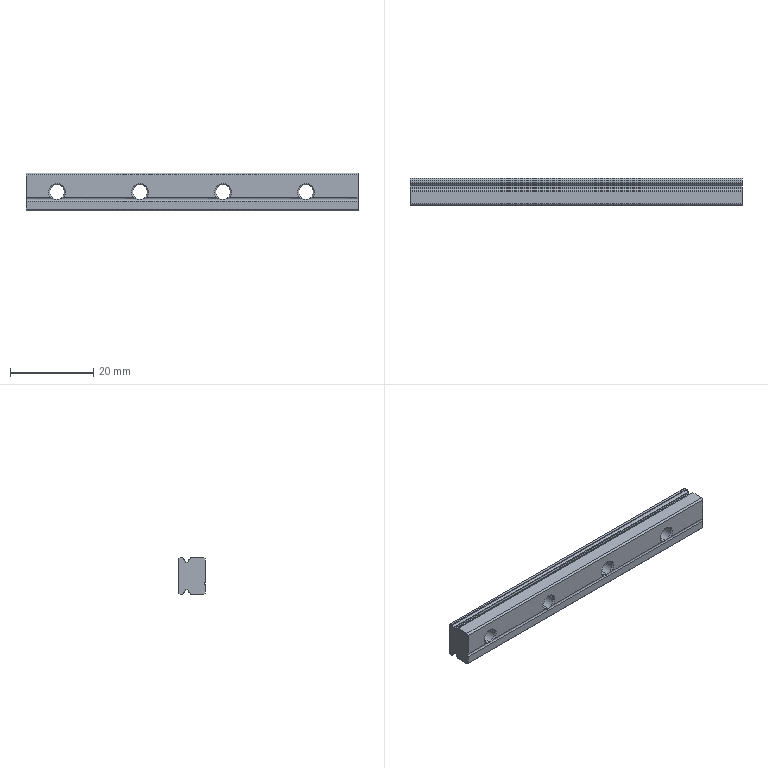Part | STEP file | 001-006-Rail_MGN9R00801HM_7_5 | 1 solid | 72 faces | box 80 x 6.5 x 9 mm | volume 3913 mm3 | cylinder 33 | plane 23 | cone 16 | commonest cylinder face diameters 0.3 x12 3.5 x8 6 x8 2 x4 1 x1